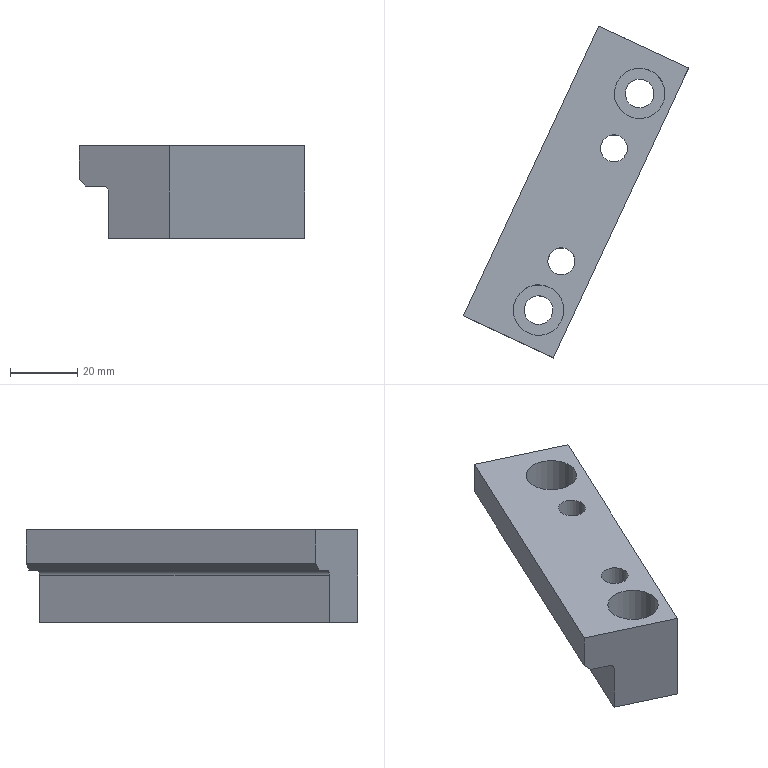Part | STEP file | gslz 2016.10.28-13_id1470_x_t | 1 solid | 18 faces | box 66.885 x 98.566 x 27.5 mm | volume 53451 mm3 | plane 11 | cylinder 7 | commonest cylinder face diameters 8 x2 8.5 x2 15 x2 3 x1
STEP:
#1=CARTESIAN_POINT('',(0.,0.,0.));
#2=DIRECTION('',(0.,0.,1.));
#3=DIRECTION('',(1.,0.,0.));
#4=AXIS2_PLACEMENT_3D('',#1,#2,#3);
#5=CARTESIAN_POINT('',(847.733,-374.977,-63.5));
#6=VERTEX_POINT('',#5);
#7=CARTESIAN_POINT('',(845.921,-374.132,-61.5));
#8=VERTEX_POINT('',#7);
#9=CARTESIAN_POINT('',(845.921,-374.132,-61.5));
#10=DIRECTION('',(-0.6409,0.2988,0.7071));
#11=VECTOR('',#10,1.);
#12=LINE('',#9,#11);
#13=CARTESIAN_POINT('',(867.052,-328.817,-61.5));
#14=DIRECTION('',(-0.6409,0.2988,-0.7071));
#15=DIRECTION('',(-0.2793,0.7673,0.5774));
#16=AXIS2_PLACEMENT_3D('',#13,#14,#15);
#17=PLANE('',#16);
#18=CARTESIAN_POINT('',(-28.868,-40.825));
#19=DIRECTION('',(0.8165,-0.5774));
#20=VECTOR('',#19,1.);
#21=LINE('',#18,#20);
#22=(GEOMETRIC_REPRESENTATION_CONTEXT(2)PARAMETRIC_REPRESENTATION_CONTEXT()REPRESENTATION_CONTEXT('',''));
#23=DEFINITIONAL_REPRESENTATION('',(#21),#22);
#24=PCURVE('',#17,#23);
#25=CARTESIAN_POINT('',(872.657,-386.599,-79.639));
#26=DIRECTION('',(0.4226,0.9063,0.));
#27=DIRECTION('',(0.9063,-0.4226,0.));
#28=AXIS2_PLACEMENT_3D('',#25,#26,#27);
#29=PLANE('',#28);
#30=CARTESIAN_POINT('',(-29.5,-18.139));
#31=DIRECTION('',(-0.7071,-0.7071));
#32=VECTOR('',#31,1.);
#33=LINE('',#30,#32);
#34=(GEOMETRIC_REPRESENTATION_CONTEXT(2)PARAMETRIC_REPRESENTATION_CONTEXT()REPRESENTATION_CONTEXT('',''));
#35=DEFINITIONAL_REPRESENTATION('',(#33),#34);
#36=PCURVE('',#29,#35);
#37=SURFACE_CURVE('',#12,(#24,#36),.PCURVE_S1.);
#38=EDGE_CURVE('',#6,#8,#37,.T.);
#39=ORIENTED_EDGE('',*,*,#38,.T.);
#40=CARTESIAN_POINT('',(886.069,-288.033,-61.5));
#41=VERTEX_POINT('',#40);
#42=CARTESIAN_POINT('',(867.052,-328.817,-61.5));
#43=DIRECTION('',(0.4226,0.9063,0.));
#44=VECTOR('',#43,1.);
#45=LINE('',#42,#44);
#46=CARTESIAN_POINT('',(0.,0.));
#47=DIRECTION('',(0.5774,0.8165));
#48=VECTOR('',#47,1.);
#49=LINE('',#46,#48);
#50=(GEOMETRIC_REPRESENTATION_CONTEXT(2)PARAMETRIC_REPRESENTATION_CONTEXT()REPRESENTATION_CONTEXT('',''));
#51=DEFINITIONAL_REPRESENTATION('',(#49),#50);
#52=PCURVE('',#17,#51);
#53=CARTESIAN_POINT('',(867.052,-328.817,-51.5));
#54=DIRECTION('',(0.9063,-0.4226,0.));
#55=DIRECTION('',(-0.4226,-0.9063,0.));
#56=AXIS2_PLACEMENT_3D('',#53,#54,#55);
#57=PLANE('',#56);
#58=CARTESIAN_POINT('',(0.,10.));
#59=DIRECTION('',(-1.,0.));
#60=VECTOR('',#59,1.);
#61=LINE('',#58,#60);
#62=(GEOMETRIC_REPRESENTATION_CONTEXT(2)PARAMETRIC_REPRESENTATION_CONTEXT()REPRESENTATION_CONTEXT('',''));
#63=DEFINITIONAL_REPRESENTATION('',(#61),#62);
#64=PCURVE('',#57,#63);
#65=SURFACE_CURVE('',#45,(#52,#64),.PCURVE_S1.);
#66=EDGE_CURVE('',#8,#41,#65,.T.);
#67=ORIENTED_EDGE('',*,*,#66,.T.);
#68=CARTESIAN_POINT('',(887.882,-288.878,-63.5));
#69=VERTEX_POINT('',#68);
#70=CARTESIAN_POINT('',(907.657,-298.1,-85.32));
#71=DIRECTION('',(0.6409,-0.2988,-0.7071));
#72=VECTOR('',#71,1.);
#73=LINE('',#70,#72);
#74=CARTESIAN_POINT('',(-1.524,56.191));
#75=DIRECTION('',(-0.8165,0.5774));
#76=VECTOR('',#75,1.);
#77=LINE('',#74,#76);
#78=(GEOMETRIC_REPRESENTATION_CONTEXT(2)PARAMETRIC_REPRESENTATION_CONTEXT()REPRESENTATION_CONTEXT('',''));
#79=DEFINITIONAL_REPRESENTATION('',(#77),#78);
#80=PCURVE('',#17,#79);
#81=CARTESIAN_POINT('',(912.805,-300.5,-79.639));
#82=DIRECTION('',(0.4226,0.9063,0.));
#83=DIRECTION('',(0.9063,-0.4226,0.));
#84=AXIS2_PLACEMENT_3D('',#81,#82,#83);
#85=PLANE('',#84);
#86=CARTESIAN_POINT('',(-5.68,5.68));
#87=DIRECTION('',(0.7071,0.7071));
#88=VECTOR('',#87,1.);
#89=LINE('',#86,#88);
#90=(GEOMETRIC_REPRESENTATION_CONTEXT(2)PARAMETRIC_REPRESENTATION_CONTEXT()REPRESENTATION_CONTEXT('',''));
#91=DEFINITIONAL_REPRESENTATION('',(#89),#90);
#92=PCURVE('',#85,#91);
#93=SURFACE_CURVE('',#73,(#80,#92),.PCURVE_S1.);
#94=EDGE_CURVE('',#41,#69,#93,.T.);
#95=ORIENTED_EDGE('',*,*,#94,.T.);
#96=CARTESIAN_POINT('',(868.864,-329.662,-63.5));
#97=DIRECTION('',(-0.4226,-0.9063,0.));
#98=VECTOR('',#97,1.);
#99=LINE('',#96,#98);
#100=CARTESIAN_POINT('',(-2.309,1.633));
#101=DIRECTION('',(-0.5774,-0.8165));
#102=VECTOR('',#101,1.);
#103=LINE('',#100,#102);
#104=(GEOMETRIC_REPRESENTATION_CONTEXT(2)PARAMETRIC_REPRESENTATION_CONTEXT()REPRESENTATION_CONTEXT('',''));
#105=DEFINITIONAL_REPRESENTATION('',(#103),#104);
#106=PCURVE('',#17,#105);
#107=CARTESIAN_POINT('',(893.788,-341.284,-63.5));
#108=DIRECTION('',(0.,0.,-1.));
#109=DIRECTION('',(-0.342,0.9397,0.));
#110=AXIS2_PLACEMENT_3D('',#107,#108,#109);
#111=PLANE('',#110);
#112=CARTESIAN_POINT('',(19.445,-19.445));
#113=DIRECTION('',(-0.7071,-0.7071));
#114=VECTOR('',#113,1.);
#115=LINE('',#112,#114);
#116=(GEOMETRIC_REPRESENTATION_CONTEXT(2)PARAMETRIC_REPRESENTATION_CONTEXT()REPRESENTATION_CONTEXT('',''));
#117=DEFINITIONAL_REPRESENTATION('',(#115),#116);
#118=PCURVE('',#111,#117);
#119=SURFACE_CURVE('',#99,(#106,#118),.PCURVE_S1.);
#120=EDGE_CURVE('',#69,#6,#119,.T.);
#121=ORIENTED_EDGE('',*,*,#120,.T.);
#122=EDGE_LOOP('',(#39,#67,#95,#121));
#123=FACE_BOUND('',#122,.T.);
#124=ADVANCED_FACE('',(#123),#17,.T.);
#125=CARTESIAN_POINT('',(893.32,-291.414,-63.5));
#126=VERTEX_POINT('',#125);
#127=CARTESIAN_POINT('',(912.805,-300.5,-63.5));
#128=DIRECTION('',(-0.9063,0.4226,0.));
#129=VECTOR('',#128,1.);
#130=LINE('',#127,#129);
#131=CARTESIAN_POINT('',(31.82,31.82));
#132=DIRECTION('',(0.7071,-0.7071));
#133=VECTOR('',#132,1.);
#134=LINE('',#131,#133);
#135=(GEOMETRIC_REPRESENTATION_CONTEXT(2)PARAMETRIC_REPRESENTATION_CONTEXT()REPRESENTATION_CONTEXT('',''));
#136=DEFINITIONAL_REPRESENTATION('',(#134),#135);
#137=PCURVE('',#111,#136);
#138=CARTESIAN_POINT('',(0.,-16.139));
#139=DIRECTION('',(-1.,0.));
#140=VECTOR('',#139,1.);
#141=LINE('',#138,#140);
#142=(GEOMETRIC_REPRESENTATION_CONTEXT(2)PARAMETRIC_REPRESENTATION_CONTEXT()REPRESENTATION_CONTEXT('',''));
#143=DEFINITIONAL_REPRESENTATION('',(#141),#142);
#144=PCURVE('',#85,#143);
#145=SURFACE_CURVE('',#130,(#137,#144),.PCURVE_S1.);
#146=EDGE_CURVE('',#126,#69,#145,.T.);
#147=ORIENTED_EDGE('',*,*,#146,.F.);
#148=CARTESIAN_POINT('',(853.171,-377.513,-63.5));
#149=VERTEX_POINT('',#148);
#150=CARTESIAN_POINT('',(874.302,-332.198,-63.5));
#151=DIRECTION('',(0.4226,0.9063,0.));
#152=VECTOR('',#151,1.);
#153=LINE('',#150,#152);
#154=CARTESIAN_POINT('',(15.203,-15.203));
#155=DIRECTION('',(0.7071,0.7071));
#156=VECTOR('',#155,1.);
#157=LINE('',#154,#156);
#158=(GEOMETRIC_REPRESENTATION_CONTEXT(2)PARAMETRIC_REPRESENTATION_CONTEXT()REPRESENTATION_CONTEXT('',''));
#159=DEFINITIONAL_REPRESENTATION('',(#157),#158);
#160=PCURVE('',#111,#159);
#161=CARTESIAN_POINT('',(874.302,-332.198,-65.));
#162=DIRECTION('',(0.4226,0.9063,0.));
#163=DIRECTION('',(0.9063,-0.4226,0.));
#164=AXIS2_PLACEMENT_3D('',#161,#162,#163);
#165=CYLINDRICAL_SURFACE('',#164,1.5);
#166=CARTESIAN_POINT('',(4.712,0.));
#167=DIRECTION('',(0.,1.));
#168=VECTOR('',#167,1.);
#169=LINE('',#166,#168);
#170=(GEOMETRIC_REPRESENTATION_CONTEXT(2)PARAMETRIC_REPRESENTATION_CONTEXT()REPRESENTATION_CONTEXT('',''));
#171=DEFINITIONAL_REPRESENTATION('',(#169),#170);
#172=PCURVE('',#165,#171);
#173=SURFACE_CURVE('',#153,(#160,#172),.PCURVE_S1.);
#174=EDGE_CURVE('',#149,#126,#173,.T.);
#175=ORIENTED_EDGE('',*,*,#174,.F.);
#176=CARTESIAN_POINT('',(872.657,-386.599,-63.5));
#177=DIRECTION('',(-0.9063,0.4226,0.));
#178=VECTOR('',#177,1.);
#179=LINE('',#176,#178);
#180=CARTESIAN_POINT('',(-35.355,-35.355));
#181=DIRECTION('',(0.7071,-0.7071));
#182=VECTOR('',#181,1.);
#183=LINE('',#180,#182);
#184=(GEOMETRIC_REPRESENTATION_CONTEXT(2)PARAMETRIC_REPRESENTATION_CONTEXT()REPRESENTATION_CONTEXT('',''));
#185=DEFINITIONAL_REPRESENTATION('',(#183),#184);
#186=PCURVE('',#111,#185);
#187=CARTESIAN_POINT('',(0.,-16.139));
#188=DIRECTION('',(-1.,0.));
#189=VECTOR('',#188,1.);
#190=LINE('',#187,#189);
#191=(GEOMETRIC_REPRESENTATION_CONTEXT(2)PARAMETRIC_REPRESENTATION_CONTEXT()REPRESENTATION_CONTEXT('',''));
#192=DEFINITIONAL_REPRESENTATION('',(#190),#191);
#193=PCURVE('',#29,#192);
#194=SURFACE_CURVE('',#179,(#186,#193),.PCURVE_S1.);
#195=EDGE_CURVE('',#149,#6,#194,.T.);
#196=ORIENTED_EDGE('',*,*,#195,.T.);
#197=ORIENTED_EDGE('',*,*,#120,.F.);
#198=EDGE_LOOP('',(#147,#175,#196,#197));
#199=FACE_BOUND('',#198,.T.);
#200=ADVANCED_FACE('',(#199),#111,.T.);
#201=CARTESIAN_POINT('',(894.679,-292.048,-65.));
#202=VERTEX_POINT('',#201);
#203=CARTESIAN_POINT('',(854.531,-378.147,-65.));
#204=VERTEX_POINT('',#203);
#205=CARTESIAN_POINT('',(875.661,-332.832,-65.));
#206=DIRECTION('',(-0.4226,-0.9063,0.));
#207=VECTOR('',#206,1.);
#208=LINE('',#205,#207);
#209=CARTESIAN_POINT('',(6.283,0.));
#210=DIRECTION('',(0.,-1.));
#211=VECTOR('',#210,1.);
#212=LINE('',#209,#211);
#213=(GEOMETRIC_REPRESENTATION_CONTEXT(2)PARAMETRIC_REPRESENTATION_CONTEXT()REPRESENTATION_CONTEXT('',''));
#214=DEFINITIONAL_REPRESENTATION('',(#212),#213);
#215=PCURVE('',#165,#214);
#216=CARTESIAN_POINT('',(875.661,-332.832,-79.639));
#217=DIRECTION('',(0.9063,-0.4226,0.));
#218=DIRECTION('',(-0.4226,-0.9063,0.));
#219=AXIS2_PLACEMENT_3D('',#216,#217,#218);
#220=PLANE('',#219);
#221=CARTESIAN_POINT('',(0.,-14.639));
#222=DIRECTION('',(1.,0.));
#223=VECTOR('',#222,1.);
#224=LINE('',#221,#223);
#225=(GEOMETRIC_REPRESENTATION_CONTEXT(2)PARAMETRIC_REPRESENTATION_CONTEXT()REPRESENTATION_CONTEXT('',''));
#226=DEFINITIONAL_REPRESENTATION('',(#224),#225);
#227=PCURVE('',#220,#226);
#228=SURFACE_CURVE('',#208,(#215,#227),.PCURVE_S1.);
#229=EDGE_CURVE('',#202,#204,#228,.T.);
#230=ORIENTED_EDGE('',*,*,#229,.F.);
#231=CARTESIAN_POINT('',(893.32,-291.414,-65.));
#232=DIRECTION('',(0.4226,0.9063,0.));
#233=DIRECTION('',(0.9063,-0.4226,0.));
#234=AXIS2_PLACEMENT_3D('',#231,#232,#233);
#235=CIRCLE('',#234,1.5);
#236=CARTESIAN_POINT('',(0.,45.));
#237=DIRECTION('',(1.,0.));
#238=VECTOR('',#237,1.);
#239=LINE('',#236,#238);
#240=(GEOMETRIC_REPRESENTATION_CONTEXT(2)PARAMETRIC_REPRESENTATION_CONTEXT()REPRESENTATION_CONTEXT('',''));
#241=DEFINITIONAL_REPRESENTATION('',(#239),#240);
#242=PCURVE('',#165,#241);
#243=CARTESIAN_POINT('',(-21.5,-14.639));
#244=DIRECTION('',(1.,0.));
#245=AXIS2_PLACEMENT_2D('',#243,#244);
#246=CIRCLE('',#245,1.5);
#247=(GEOMETRIC_REPRESENTATION_CONTEXT(2)PARAMETRIC_REPRESENTATION_CONTEXT()REPRESENTATION_CONTEXT('',''));
#248=DEFINITIONAL_REPRESENTATION('',(#246),#247);
#249=PCURVE('',#85,#248);
#250=SURFACE_CURVE('',#235,(#242,#249),.PCURVE_S1.);
#251=EDGE_CURVE('',#126,#202,#250,.T.);
#252=ORIENTED_EDGE('',*,*,#251,.F.);
#253=ORIENTED_EDGE('',*,*,#174,.F.);
#254=CARTESIAN_POINT('',(853.171,-377.513,-65.));
#255=DIRECTION('',(-0.4226,-0.9063,0.));
#256=DIRECTION('',(0.9063,-0.4226,0.));
#257=AXIS2_PLACEMENT_3D('',#254,#255,#256);
#258=CIRCLE('',#257,1.5);
#259=CARTESIAN_POINT('',(6.283,-50.));
#260=DIRECTION('',(-1.,0.));
#261=VECTOR('',#260,1.);
#262=LINE('',#259,#261);
#263=(GEOMETRIC_REPRESENTATION_CONTEXT(2)PARAMETRIC_REPRESENTATION_CONTEXT()REPRESENTATION_CONTEXT('',''));
#264=DEFINITIONAL_REPRESENTATION('',(#262),#263);
#265=PCURVE('',#165,#264);
#266=CARTESIAN_POINT('',(-20.,-14.639));
#267=CARTESIAN_POINT('',(-20.,-17.237));
#268=CARTESIAN_POINT('',(-22.25,-15.938));
#269=CARTESIAN_POINT('',(-24.5,-14.639));
#270=CARTESIAN_POINT('',(-22.25,-13.34));
#271=CARTESIAN_POINT('',(-20.,-12.041));
#272=CARTESIAN_POINT('',(-20.,-14.639));
#273=(BOUNDED_CURVE()B_SPLINE_CURVE(2,(#266,#267,#268,#269,#270,#271,#272),.UNSPECIFIED.,.T.,.F.)B_SPLINE_CURVE_WITH_KNOTS((1,2,2,2,2,1),(-2.094,0.,2.094,4.189,6.283,8.378),.UNSPECIFIED.)CURVE()GEOMETRIC_REPRESENTATION_ITEM()RATIONAL_B_SPLINE_CURVE((1.,0.5,1.,0.5,1.,0.5,1.))REPRESENTATION_ITEM(''));
#274=(GEOMETRIC_REPRESENTATION_CONTEXT(2)PARAMETRIC_REPRESENTATION_CONTEXT()REPRESENTATION_CONTEXT('',''));
#275=DEFINITIONAL_REPRESENTATION('',(#273),#274);
#276=PCURVE('',#29,#275);
#277=SURFACE_CURVE('',#258,(#265,#276),.PCURVE_S1.);
#278=EDGE_CURVE('',#204,#149,#277,.T.);
#279=ORIENTED_EDGE('',*,*,#278,.F.);
#280=EDGE_LOOP('',(#230,#252,#253,#279));
#281=FACE_BOUND('',#280,.F.);
#282=ADVANCED_FACE('',(#281),#165,.F.);
#283=CARTESIAN_POINT('',(896.795,-304.062,-66.5));
#284=VERTEX_POINT('',#283);
#285=CARTESIAN_POINT('',(898.248,-308.056,-66.5));
#286=DIRECTION('',(0.,0.,-1.));
#287=DIRECTION('',(-0.342,0.9397,0.));
#288=AXIS2_PLACEMENT_3D('',#285,#286,#287);
#289=CIRCLE('',#288,4.25);
#290=CARTESIAN_POINT('',(898.248,-308.056,-66.5));
#291=DIRECTION('',(0.,0.,-1.));
#292=DIRECTION('',(-0.342,0.9397,0.));
#293=AXIS2_PLACEMENT_3D('',#290,#291,#292);
#294=PLANE('',#293);
#295=CARTESIAN_POINT('',(0.,0.));
#296=DIRECTION('',(1.,0.));
#297=AXIS2_PLACEMENT_2D('',#295,#296);
#298=CIRCLE('',#297,4.25);
#299=(GEOMETRIC_REPRESENTATION_CONTEXT(2)PARAMETRIC_REPRESENTATION_CONTEXT()REPRESENTATION_CONTEXT('',''));
#300=DEFINITIONAL_REPRESENTATION('',(#298),#299);
#301=PCURVE('',#294,#300);
#302=CARTESIAN_POINT('',(898.248,-308.056,-101.5));
#303=DIRECTION('',(0.,0.,-1.));
#304=DIRECTION('',(-0.342,0.9397,0.));
#305=AXIS2_PLACEMENT_3D('',#302,#303,#304);
#306=CYLINDRICAL_SURFACE('',#305,4.25);
#307=CARTESIAN_POINT('',(0.,-35.));
#308=DIRECTION('',(1.,0.));
#309=VECTOR('',#308,1.);
#310=LINE('',#307,#309);
#311=(GEOMETRIC_REPRESENTATION_CONTEXT(2)PARAMETRIC_REPRESENTATION_CONTEXT()REPRESENTATION_CONTEXT('',''));
#312=DEFINITIONAL_REPRESENTATION('',(#310),#311);
#313=PCURVE('',#306,#312);
#314=SURFACE_CURVE('',#289,(#301,#313),.PCURVE_S1.);
#315=EDGE_CURVE('',#284,#284,#314,.T.);
#316=ORIENTED_EDGE('',*,*,#315,.T.);
#317=EDGE_LOOP('',(#316));
#318=FACE_BOUND('',#317,.T.);
#319=CARTESIAN_POINT('',(895.683,-301.008,-66.5));
#320=VERTEX_POINT('',#319);
#321=CARTESIAN_POINT('',(898.248,-308.056,-66.5));
#322=DIRECTION('',(0.,0.,-1.));
#323=DIRECTION('',(-0.342,0.9397,0.));
#324=AXIS2_PLACEMENT_3D('',#321,#322,#323);
#325=CIRCLE('',#324,7.5);
#326=CARTESIAN_POINT('',(0.,0.));
#327=DIRECTION('',(1.,0.));
#328=AXIS2_PLACEMENT_2D('',#326,#327);
#329=CIRCLE('',#328,7.5);
#330=(GEOMETRIC_REPRESENTATION_CONTEXT(2)PARAMETRIC_REPRESENTATION_CONTEXT()REPRESENTATION_CONTEXT('',''));
#331=DEFINITIONAL_REPRESENTATION('',(#329),#330);
#332=PCURVE('',#294,#331);
#333=CARTESIAN_POINT('',(898.248,-308.056,-51.5));
#334=DIRECTION('',(0.,0.,-1.));
#335=DIRECTION('',(-0.342,0.9397,0.));
#336=AXIS2_PLACEMENT_3D('',#333,#334,#335);
#337=CYLINDRICAL_SURFACE('',#336,7.5);
#338=CARTESIAN_POINT('',(0.,15.));
#339=DIRECTION('',(1.,0.));
#340=VECTOR('',#339,1.);
#341=LINE('',#338,#340);
#342=(GEOMETRIC_REPRESENTATION_CONTEXT(2)PARAMETRIC_REPRESENTATION_CONTEXT()REPRESENTATION_CONTEXT('',''));
#343=DEFINITIONAL_REPRESENTATION('',(#341),#342);
#344=PCURVE('',#337,#343);
#345=SURFACE_CURVE('',#325,(#332,#344),.PCURVE_S1.);
#346=EDGE_CURVE('',#320,#320,#345,.T.);
#347=ORIENTED_EDGE('',*,*,#346,.F.);
#348=EDGE_LOOP('',(#347));
#349=FACE_BOUND('',#348,.T.);
#350=ADVANCED_FACE('',(#318,#349),#294,.F.);
#351=CARTESIAN_POINT('',(866.789,-368.41,-66.5));
#352=VERTEX_POINT('',#351);
#353=CARTESIAN_POINT('',(868.242,-372.404,-66.5));
#354=DIRECTION('',(0.,0.,-1.));
#355=DIRECTION('',(-0.342,0.9397,0.));
#356=AXIS2_PLACEMENT_3D('',#353,#354,#355);
#357=CIRCLE('',#356,4.25);
#358=CARTESIAN_POINT('',(874.582,-358.809,-66.5));
#359=DIRECTION('',(0.,0.,-1.));
#360=DIRECTION('',(-0.342,0.9397,0.));
#361=AXIS2_PLACEMENT_3D('',#358,#359,#360);
#362=PLANE('',#361);
#363=CARTESIAN_POINT('',(-10.607,-10.607));
#364=DIRECTION('',(1.,0.));
#365=AXIS2_PLACEMENT_2D('',#363,#364);
#366=CIRCLE('',#365,4.25);
#367=(GEOMETRIC_REPRESENTATION_CONTEXT(2)PARAMETRIC_REPRESENTATION_CONTEXT()REPRESENTATION_CONTEXT('',''));
#368=DEFINITIONAL_REPRESENTATION('',(#366),#367);
#369=PCURVE('',#362,#368);
#370=CARTESIAN_POINT('',(868.242,-372.404,-101.5));
#371=DIRECTION('',(0.,0.,-1.));
#372=DIRECTION('',(-0.342,0.9397,0.));
#373=AXIS2_PLACEMENT_3D('',#370,#371,#372);
#374=CYLINDRICAL_SURFACE('',#373,4.25);
#375=CARTESIAN_POINT('',(0.,-35.));
#376=DIRECTION('',(1.,0.));
#377=VECTOR('',#376,1.);
#378=LINE('',#375,#377);
#379=(GEOMETRIC_REPRESENTATION_CONTEXT(2)PARAMETRIC_REPRESENTATION_CONTEXT()REPRESENTATION_CONTEXT('',''));
#380=DEFINITIONAL_REPRESENTATION('',(#378),#379);
#381=PCURVE('',#374,#380);
#382=SURFACE_CURVE('',#357,(#369,#381),.PCURVE_S1.);
#383=EDGE_CURVE('',#352,#352,#382,.T.);
#384=ORIENTED_EDGE('',*,*,#383,.T.);
#385=EDGE_LOOP('',(#384));
#386=FACE_BOUND('',#385,.T.);
#387=CARTESIAN_POINT('',(865.677,-365.356,-66.5));
#388=VERTEX_POINT('',#387);
#389=CARTESIAN_POINT('',(868.242,-372.404,-66.5));
#390=DIRECTION('',(0.,0.,-1.));
#391=DIRECTION('',(-0.342,0.9397,0.));
#392=AXIS2_PLACEMENT_3D('',#389,#390,#391);
#393=CIRCLE('',#392,7.5);
#394=CARTESIAN_POINT('',(-10.607,-10.607));
#395=DIRECTION('',(1.,0.));
#396=AXIS2_PLACEMENT_2D('',#394,#395);
#397=CIRCLE('',#396,7.5);
#398=(GEOMETRIC_REPRESENTATION_CONTEXT(2)PARAMETRIC_REPRESENTATION_CONTEXT()REPRESENTATION_CONTEXT('',''));
#399=DEFINITIONAL_REPRESENTATION('',(#397),#398);
#400=PCURVE('',#362,#399);
#401=CARTESIAN_POINT('',(868.242,-372.404,-51.5));
#402=DIRECTION('',(0.,0.,-1.));
#403=DIRECTION('',(-0.342,0.9397,0.));
#404=AXIS2_PLACEMENT_3D('',#401,#402,#403);
#405=CYLINDRICAL_SURFACE('',#404,7.5);
#406=CARTESIAN_POINT('',(0.,15.));
#407=DIRECTION('',(1.,0.));
#408=VECTOR('',#407,1.);
#409=LINE('',#406,#408);
#410=(GEOMETRIC_REPRESENTATION_CONTEXT(2)PARAMETRIC_REPRESENTATION_CONTEXT()REPRESENTATION_CONTEXT('',''));
#411=DEFINITIONAL_REPRESENTATION('',(#409),#410);
#412=PCURVE('',#405,#411);
#413=SURFACE_CURVE('',#393,(#400,#412),.PCURVE_S1.);
#414=EDGE_CURVE('',#388,#388,#413,.T.);
#415=ORIENTED_EDGE('',*,*,#414,.F.);
#416=EDGE_LOOP('',(#415));
#417=FACE_BOUND('',#416,.T.);
#418=ADVANCED_FACE('',(#386,#417),#362,.F.);
#419=CARTESIAN_POINT('',(886.069,-288.033,-51.5));
#420=VERTEX_POINT('',#419);
#421=CARTESIAN_POINT('',(886.069,-288.033,-51.5));
#422=DIRECTION('',(0.,0.,-1.));
#423=VECTOR('',#422,1.);
#424=LINE('',#421,#423);
#425=CARTESIAN_POINT('',(-45.,0.));
#426=DIRECTION('',(0.,1.));
#427=VECTOR('',#426,1.);
#428=LINE('',#425,#427);
#429=(GEOMETRIC_REPRESENTATION_CONTEXT(2)PARAMETRIC_REPRESENTATION_CONTEXT()REPRESENTATION_CONTEXT('',''));
#430=DEFINITIONAL_REPRESENTATION('',(#428),#429);
#431=PCURVE('',#57,#430);
#432=CARTESIAN_POINT('',(-29.5,-28.139));
#433=DIRECTION('',(0.,1.));
#434=VECTOR('',#433,1.);
#435=LINE('',#432,#434);
#436=(GEOMETRIC_REPRESENTATION_CONTEXT(2)PARAMETRIC_REPRESENTATION_CONTEXT()REPRESENTATION_CONTEXT('',''));
#437=DEFINITIONAL_REPRESENTATION('',(#435),#436);
#438=PCURVE('',#85,#437);
#439=SURFACE_CURVE('',#424,(#431,#438),.PCURVE_S1.);
#440=EDGE_CURVE('',#420,#41,#439,.T.);
#441=ORIENTED_EDGE('',*,*,#440,.T.);
#442=ORIENTED_EDGE('',*,*,#66,.F.);
#443=CARTESIAN_POINT('',(845.921,-374.132,-51.5));
#444=VERTEX_POINT('',#443);
#445=CARTESIAN_POINT('',(845.921,-374.132,-51.5));
#446=DIRECTION('',(0.,0.,-1.));
#447=VECTOR('',#446,1.);
#448=LINE('',#445,#447);
#449=CARTESIAN_POINT('',(50.,0.));
#450=DIRECTION('',(0.,1.));
#451=VECTOR('',#450,1.);
#452=LINE('',#449,#451);
#453=(GEOMETRIC_REPRESENTATION_CONTEXT(2)PARAMETRIC_REPRESENTATION_CONTEXT()REPRESENTATION_CONTEXT('',''));
#454=DEFINITIONAL_REPRESENTATION('',(#452),#453);
#455=PCURVE('',#57,#454);
#456=CARTESIAN_POINT('',(-29.5,-28.139));
#457=DIRECTION('',(0.,1.));
#458=VECTOR('',#457,1.);
#459=LINE('',#456,#458);
#460=(GEOMETRIC_REPRESENTATION_CONTEXT(2)PARAMETRIC_REPRESENTATION_CONTEXT()REPRESENTATION_CONTEXT('',''));
#461=DEFINITIONAL_REPRESENTATION('',(#459),#460);
#462=PCURVE('',#29,#461);
#463=SURFACE_CURVE('',#448,(#455,#462),.PCURVE_S1.);
#464=EDGE_CURVE('',#444,#8,#463,.T.);
#465=ORIENTED_EDGE('',*,*,#464,.F.);
#466=CARTESIAN_POINT('',(867.052,-328.817,-51.5));
#467=DIRECTION('',(-0.4226,-0.9063,0.));
#468=VECTOR('',#467,1.);
#469=LINE('',#466,#468);
#470=CARTESIAN_POINT('',(0.,0.));
#471=DIRECTION('',(1.,0.));
#472=VECTOR('',#471,1.);
#473=LINE('',#470,#472);
#474=(GEOMETRIC_REPRESENTATION_CONTEXT(2)PARAMETRIC_REPRESENTATION_CONTEXT()REPRESENTATION_CONTEXT('',''));
#475=DEFINITIONAL_REPRESENTATION('',(#473),#474);
#476=PCURVE('',#57,#475);
#477=CARTESIAN_POINT('',(893.788,-341.284,-51.5));
#478=DIRECTION('',(0.,0.,-1.));
#479=DIRECTION('',(-0.342,0.9397,0.));
#480=AXIS2_PLACEMENT_3D('',#477,#478,#479);
#481=PLANE('',#480);
#482=CARTESIAN_POINT('',(20.86,-20.86));
#483=DIRECTION('',(-0.7071,-0.7071));
#484=VECTOR('',#483,1.);
#485=LINE('',#482,#484);
#486=(GEOMETRIC_REPRESENTATION_CONTEXT(2)PARAMETRIC_REPRESENTATION_CONTEXT()REPRESENTATION_CONTEXT('',''));
#487=DEFINITIONAL_REPRESENTATION('',(#485),#486);
#488=PCURVE('',#481,#487);
#489=SURFACE_CURVE('',#469,(#476,#488),.PCURVE_S1.);
#490=EDGE_CURVE('',#420,#444,#489,.T.);
#491=ORIENTED_EDGE('',*,*,#490,.F.);
#492=EDGE_LOOP('',(#441,#442,#465,#491));
#493=FACE_BOUND('',#492,.T.);
#494=ADVANCED_FACE('',(#493),#57,.F.);
#495=ORIENTED_EDGE('',*,*,#346,.F.);
#496=CARTESIAN_POINT('',(895.683,-301.008,-51.5));
#497=VERTEX_POINT('',#496);
#498=CARTESIAN_POINT('',(895.683,-301.008,-51.5));
#499=CARTESIAN_POINT('',(895.683,-301.008,-66.5));
#500=B_SPLINE_CURVE_WITH_KNOTS('',1,(#498,#499),.UNSPECIFIED.,.F.,.F.,(2,2),(0.,15.),.PIECEWISE_BEZIER_KNOTS.);
#501=CARTESIAN_POINT('',(0.,0.));
#502=DIRECTION('',(0.,1.));
#503=VECTOR('',#502,1.);
#504=LINE('',#501,#503);
#505=(GEOMETRIC_REPRESENTATION_CONTEXT(2)PARAMETRIC_REPRESENTATION_CONTEXT()REPRESENTATION_CONTEXT('',''));
#506=DEFINITIONAL_REPRESENTATION('',(#504),#505);
#507=PCURVE('',#337,#506);
#508=CARTESIAN_POINT('',(6.283,0.));
#509=DIRECTION('',(0.,1.));
#510=VECTOR('',#509,1.);
#511=LINE('',#508,#510);
#512=(GEOMETRIC_REPRESENTATION_CONTEXT(2)PARAMETRIC_REPRESENTATION_CONTEXT()REPRESENTATION_CONTEXT('',''));
#513=DEFINITIONAL_REPRESENTATION('',(#511),#512);
#514=PCURVE('',#337,#513);
#515=SEAM_CURVE('',#500,(#507,#514),.PCURVE_S1.);
#516=EDGE_CURVE('',#497,#320,#515,.T.);
#517=ORIENTED_EDGE('',*,*,#516,.F.);
#518=CARTESIAN_POINT('',(898.248,-308.056,-51.5));
#519=DIRECTION('',(0.,0.,1.));
#520=DIRECTION('',(-0.342,0.9397,0.));
#521=AXIS2_PLACEMENT_3D('',#518,#519,#520);
#522=CIRCLE('',#521,7.5);
#523=CARTESIAN_POINT('',(6.283,0.));
#524=DIRECTION('',(-1.,0.));
#525=VECTOR('',#524,1.);
#526=LINE('',#523,#525);
#527=(GEOMETRIC_REPRESENTATION_CONTEXT(2)PARAMETRIC_REPRESENTATION_CONTEXT()REPRESENTATION_CONTEXT('',''));
#528=DEFINITIONAL_REPRESENTATION('',(#526),#527);
#529=PCURVE('',#337,#528);
#530=CARTESIAN_POINT('',(37.198,15.556));
#531=CARTESIAN_POINT('',(37.198,2.566));
#532=CARTESIAN_POINT('',(25.948,9.061));
#533=CARTESIAN_POINT('',(14.698,15.556));
#534=CARTESIAN_POINT('',(25.948,22.052));
#535=CARTESIAN_POINT('',(37.198,28.547));
#536=CARTESIAN_POINT('',(37.198,15.556));
#537=(BOUNDED_CURVE()B_SPLINE_CURVE(2,(#530,#531,#532,#533,#534,#535,#536),.UNSPECIFIED.,.T.,.F.)B_SPLINE_CURVE_WITH_KNOTS((1,2,2,2,2,1),(-2.094,0.,2.094,4.189,6.283,8.378),.UNSPECIFIED.)CURVE()GEOMETRIC_REPRESENTATION_ITEM()RATIONAL_B_SPLINE_CURVE((1.,0.5,1.,0.5,1.,0.5,1.))REPRESENTATION_ITEM(''));
#538=(GEOMETRIC_REPRESENTATION_CONTEXT(2)PARAMETRIC_REPRESENTATION_CONTEXT()REPRESENTATION_CONTEXT('',''));
#539=DEFINITIONAL_REPRESENTATION('',(#537),#538);
#540=PCURVE('',#481,#539);
#541=SURFACE_CURVE('',#522,(#529,#540),.PCURVE_S1.);
#542=EDGE_CURVE('',#497,#497,#541,.T.);
#543=ORIENTED_EDGE('',*,*,#542,.F.);
#544=ORIENTED_EDGE('',*,*,#516,.T.);
#545=EDGE_LOOP('',(#495,#517,#543,#544));
#546=FACE_BOUND('',#545,.F.);
#547=ADVANCED_FACE('',(#546),#337,.F.);
#548=ORIENTED_EDGE('',*,*,#414,.F.);
#549=CARTESIAN_POINT('',(865.677,-365.356,-51.5));
#550=VERTEX_POINT('',#549);
#551=CARTESIAN_POINT('',(865.677,-365.356,-51.5));
#552=CARTESIAN_POINT('',(865.677,-365.356,-66.5));
#553=B_SPLINE_CURVE_WITH_KNOTS('',1,(#551,#552),.UNSPECIFIED.,.F.,.F.,(2,2),(0.,15.),.PIECEWISE_BEZIER_KNOTS.);
#554=CARTESIAN_POINT('',(0.,0.));
#555=DIRECTION('',(0.,1.));
#556=VECTOR('',#555,1.);
#557=LINE('',#554,#556);
#558=(GEOMETRIC_REPRESENTATION_CONTEXT(2)PARAMETRIC_REPRESENTATION_CONTEXT()REPRESENTATION_CONTEXT('',''));
#559=DEFINITIONAL_REPRESENTATION('',(#557),#558);
#560=PCURVE('',#405,#559);
#561=CARTESIAN_POINT('',(6.283,0.));
#562=DIRECTION('',(0.,1.));
#563=VECTOR('',#562,1.);
#564=LINE('',#561,#563);
#565=(GEOMETRIC_REPRESENTATION_CONTEXT(2)PARAMETRIC_REPRESENTATION_CONTEXT()REPRESENTATION_CONTEXT('',''));
#566=DEFINITIONAL_REPRESENTATION('',(#564),#565);
#567=PCURVE('',#405,#566);
#568=SEAM_CURVE('',#553,(#560,#567),.PCURVE_S1.);
#569=EDGE_CURVE('',#550,#388,#568,.T.);
#570=ORIENTED_EDGE('',*,*,#569,.F.);
#571=CARTESIAN_POINT('',(868.242,-372.404,-51.5));
#572=DIRECTION('',(0.,0.,1.));
#573=DIRECTION('',(-0.342,0.9397,0.));
#574=AXIS2_PLACEMENT_3D('',#571,#572,#573);
#575=CIRCLE('',#574,7.5);
#576=CARTESIAN_POINT('',(6.283,0.));
#577=DIRECTION('',(-1.,0.));
#578=VECTOR('',#577,1.);
#579=LINE('',#576,#578);
#580=(GEOMETRIC_REPRESENTATION_CONTEXT(2)PARAMETRIC_REPRESENTATION_CONTEXT()REPRESENTATION_CONTEXT('',''));
#581=DEFINITIONAL_REPRESENTATION('',(#579),#580);
#582=PCURVE('',#405,#581);
#583=CARTESIAN_POINT('',(-13.006,-34.648));
#584=CARTESIAN_POINT('',(-13.006,-47.639));
#585=CARTESIAN_POINT('',(-24.256,-41.143));
#586=CARTESIAN_POINT('',(-35.506,-34.648));
#587=CARTESIAN_POINT('',(-24.256,-28.153));
#588=CARTESIAN_POINT('',(-13.006,-21.658));
#589=CARTESIAN_POINT('',(-13.006,-34.648));
#590=(BOUNDED_CURVE()B_SPLINE_CURVE(2,(#583,#584,#585,#586,#587,#588,#589),.UNSPECIFIED.,.T.,.F.)B_SPLINE_CURVE_WITH_KNOTS((1,2,2,2,2,1),(-2.094,0.,2.094,4.189,6.283,8.378),.UNSPECIFIED.)CURVE()GEOMETRIC_REPRESENTATION_ITEM()RATIONAL_B_SPLINE_CURVE((1.,0.5,1.,0.5,1.,0.5,1.))REPRESENTATION_ITEM(''));
#591=(GEOMETRIC_REPRESENTATION_CONTEXT(2)PARAMETRIC_REPRESENTATION_CONTEXT()REPRESENTATION_CONTEXT('',''));
#592=DEFINITIONAL_REPRESENTATION('',(#590),#591);
#593=PCURVE('',#481,#592);
#594=SURFACE_CURVE('',#575,(#582,#593),.PCURVE_S1.);
#595=EDGE_CURVE('',#550,#550,#594,.T.);
#596=ORIENTED_EDGE('',*,*,#595,.F.);
#597=ORIENTED_EDGE('',*,*,#569,.T.);
#598=EDGE_LOOP('',(#548,#570,#596,#597));
#599=FACE_BOUND('',#598,.F.);
#600=ADVANCED_FACE('',(#599),#405,.F.);
#601=CARTESIAN_POINT('',(912.805,-300.5,-51.5));
#602=VERTEX_POINT('',#601);
#603=CARTESIAN_POINT('',(912.805,-300.5,-51.5));
#604=DIRECTION('',(-0.9063,0.4226,0.));
#605=VECTOR('',#604,1.);
#606=LINE('',#603,#605);
#607=CARTESIAN_POINT('',(0.,-28.139));
#608=DIRECTION('',(-1.,0.));
#609=VECTOR('',#608,1.);
#610=LINE('',#607,#609);
#611=(GEOMETRIC_REPRESENTATION_CONTEXT(2)PARAMETRIC_REPRESENTATION_CONTEXT()REPRESENTATION_CONTEXT('',''));
#612=DEFINITIONAL_REPRESENTATION('',(#610),#611);
#613=PCURVE('',#85,#612);
#614=CARTESIAN_POINT('',(31.82,31.82));
#615=DIRECTION('',(0.7071,-0.7071));
#616=VECTOR('',#615,1.);
#617=LINE('',#614,#616);
#618=(GEOMETRIC_REPRESENTATION_CONTEXT(2)PARAMETRIC_REPRESENTATION_CONTEXT()REPRESENTATION_CONTEXT('',''));
#619=DEFINITIONAL_REPRESENTATION('',(#617),#618);
#620=PCURVE('',#481,#619);
#621=SURFACE_CURVE('',#606,(#613,#620),.PCURVE_S1.);
#622=EDGE_CURVE('',#602,#420,#621,.T.);
#623=ORIENTED_EDGE('',*,*,#622,.F.);
#624=CARTESIAN_POINT('',(912.805,-300.5,-79.));
#625=VERTEX_POINT('',#624);
#626=CARTESIAN_POINT('',(912.805,-300.5,-79.639));
#627=DIRECTION('',(0.,0.,1.));
#628=VECTOR('',#627,1.);
#629=LINE('',#626,#628);
#630=CARTESIAN_POINT('',(0.,0.));
#631=DIRECTION('',(0.,-1.));
#632=VECTOR('',#631,1.);
#633=LINE('',#630,#632);
#634=(GEOMETRIC_REPRESENTATION_CONTEXT(2)PARAMETRIC_REPRESENTATION_CONTEXT()REPRESENTATION_CONTEXT('',''));
#635=DEFINITIONAL_REPRESENTATION('',(#633),#634);
#636=PCURVE('',#85,#635);
#637=CARTESIAN_POINT('',(893.788,-341.284,-79.639));
#638=DIRECTION('',(0.9063,-0.4226,0.));
#639=DIRECTION('',(-0.4226,-0.9063,0.));
#640=AXIS2_PLACEMENT_3D('',#637,#638,#639);
#641=PLANE('',#640);
#642=CARTESIAN_POINT('',(-45.,0.));
#643=DIRECTION('',(0.,-1.));
#644=VECTOR('',#643,1.);
#645=LINE('',#642,#644);
#646=(GEOMETRIC_REPRESENTATION_CONTEXT(2)PARAMETRIC_REPRESENTATION_CONTEXT()REPRESENTATION_CONTEXT('',''));
#647=DEFINITIONAL_REPRESENTATION('',(#645),#646);
#648=PCURVE('',#641,#647);
#649=SURFACE_CURVE('',#629,(#636,#648),.PCURVE_S1.);
#650=EDGE_CURVE('',#625,#602,#649,.T.);
#651=ORIENTED_EDGE('',*,*,#650,.F.);
#652=CARTESIAN_POINT('',(894.679,-292.048,-79.));
#653=VERTEX_POINT('',#652);
#654=CARTESIAN_POINT('',(912.805,-300.5,-79.));
#655=DIRECTION('',(-0.9063,0.4226,0.));
#656=VECTOR('',#655,1.);
#657=LINE('',#654,#656);
#658=CARTESIAN_POINT('',(0.,-0.6394));
#659=DIRECTION('',(-1.,0.));
#660=VECTOR('',#659,1.);
#661=LINE('',#658,#660);
#662=(GEOMETRIC_REPRESENTATION_CONTEXT(2)PARAMETRIC_REPRESENTATION_CONTEXT()REPRESENTATION_CONTEXT('',''));
#663=DEFINITIONAL_REPRESENTATION('',(#661),#662);
#664=PCURVE('',#85,#663);
#665=CARTESIAN_POINT('',(893.788,-341.284,-79.));
#666=DIRECTION('',(0.,0.,-1.));
#667=DIRECTION('',(-0.342,0.9397,0.));
#668=AXIS2_PLACEMENT_3D('',#665,#666,#667);
#669=PLANE('',#668);
#670=CARTESIAN_POINT('',(31.82,31.82));
#671=DIRECTION('',(0.7071,-0.7071));
#672=VECTOR('',#671,1.);
#673=LINE('',#670,#672);
#674=(GEOMETRIC_REPRESENTATION_CONTEXT(2)PARAMETRIC_REPRESENTATION_CONTEXT()REPRESENTATION_CONTEXT('',''));
#675=DEFINITIONAL_REPRESENTATION('',(#673),#674);
#676=PCURVE('',#669,#675);
#677=SURFACE_CURVE('',#657,(#664,#676),.PCURVE_S1.);
#678=EDGE_CURVE('',#625,#653,#677,.T.);
#679=ORIENTED_EDGE('',*,*,#678,.T.);
#680=CARTESIAN_POINT('',(894.679,-292.048,-79.639));
#681=DIRECTION('',(0.,0.,1.));
#682=VECTOR('',#681,1.);
#683=LINE('',#680,#682);
#684=CARTESIAN_POINT('',(-20.,0.));
#685=DIRECTION('',(0.,-1.));
#686=VECTOR('',#685,1.);
#687=LINE('',#684,#686);
#688=(GEOMETRIC_REPRESENTATION_CONTEXT(2)PARAMETRIC_REPRESENTATION_CONTEXT()REPRESENTATION_CONTEXT('',''));
#689=DEFINITIONAL_REPRESENTATION('',(#687),#688);
#690=PCURVE('',#85,#689);
#691=CARTESIAN_POINT('',(-45.,0.));
#692=DIRECTION('',(0.,-1.));
#693=VECTOR('',#692,1.);
#694=LINE('',#691,#693);
#695=(GEOMETRIC_REPRESENTATION_CONTEXT(2)PARAMETRIC_REPRESENTATION_CONTEXT()REPRESENTATION_CONTEXT('',''));
#696=DEFINITIONAL_REPRESENTATION('',(#694),#695);
#697=PCURVE('',#220,#696);
#698=SURFACE_CURVE('',#683,(#690,#697),.PCURVE_S1.);
#699=EDGE_CURVE('',#653,#202,#698,.T.);
#700=ORIENTED_EDGE('',*,*,#699,.T.);
#701=ORIENTED_EDGE('',*,*,#251,.F.);
#702=ORIENTED_EDGE('',*,*,#146,.T.);
#703=ORIENTED_EDGE('',*,*,#94,.F.);
#704=ORIENTED_EDGE('',*,*,#440,.F.);
#705=EDGE_LOOP('',(#623,#651,#679,#700,#701,#702,#703,#704));
#706=FACE_BOUND('',#705,.T.);
#707=ADVANCED_FACE('',(#706),#85,.T.);
#708=CARTESIAN_POINT('',(872.657,-386.599,-79.));
#709=VERTEX_POINT('',#708);
#710=CARTESIAN_POINT('',(872.657,-386.599,-51.5));
#711=VERTEX_POINT('',#710);
#712=CARTESIAN_POINT('',(872.657,-386.599,-79.639));
#713=DIRECTION('',(0.,0.,1.));
#714=VECTOR('',#713,1.);
#715=LINE('',#712,#714);
#716=CARTESIAN_POINT('',(50.,0.));
#717=DIRECTION('',(0.,-1.));
#718=VECTOR('',#717,1.);
#719=LINE('',#716,#718);
#720=(GEOMETRIC_REPRESENTATION_CONTEXT(2)PARAMETRIC_REPRESENTATION_CONTEXT()REPRESENTATION_CONTEXT('',''));
#721=DEFINITIONAL_REPRESENTATION('',(#719),#720);
#722=PCURVE('',#641,#721);
#723=CARTESIAN_POINT('',(0.,0.));
#724=DIRECTION('',(0.,-1.));
#725=VECTOR('',#724,1.);
#726=LINE('',#723,#725);
#727=(GEOMETRIC_REPRESENTATION_CONTEXT(2)PARAMETRIC_REPRESENTATION_CONTEXT()REPRESENTATION_CONTEXT('',''));
#728=DEFINITIONAL_REPRESENTATION('',(#726),#727);
#729=PCURVE('',#29,#728);
#730=SURFACE_CURVE('',#715,(#722,#729),.PCURVE_S1.);
#731=EDGE_CURVE('',#709,#711,#730,.T.);
#732=ORIENTED_EDGE('',*,*,#731,.F.);
#733=CARTESIAN_POINT('',(893.788,-341.284,-79.));
#734=DIRECTION('',(0.4226,0.9063,0.));
#735=VECTOR('',#734,1.);
#736=LINE('',#733,#735);
#737=CARTESIAN_POINT('',(0.,-0.6394));
#738=DIRECTION('',(-1.,0.));
#739=VECTOR('',#738,1.);
#740=LINE('',#737,#739);
#741=(GEOMETRIC_REPRESENTATION_CONTEXT(2)PARAMETRIC_REPRESENTATION_CONTEXT()REPRESENTATION_CONTEXT('',''));
#742=DEFINITIONAL_REPRESENTATION('',(#740),#741);
#743=PCURVE('',#641,#742);
#744=CARTESIAN_POINT('',(0.,0.));
#745=DIRECTION('',(0.7071,0.7071));
#746=VECTOR('',#745,1.);
#747=LINE('',#744,#746);
#748=(GEOMETRIC_REPRESENTATION_CONTEXT(2)PARAMETRIC_REPRESENTATION_CONTEXT()REPRESENTATION_CONTEXT('',''));
#749=DEFINITIONAL_REPRESENTATION('',(#747),#748);
#750=PCURVE('',#669,#749);
#751=SURFACE_CURVE('',#736,(#743,#750),.PCURVE_S1.);
#752=EDGE_CURVE('',#709,#625,#751,.T.);
#753=ORIENTED_EDGE('',*,*,#752,.T.);
#754=ORIENTED_EDGE('',*,*,#650,.T.);
#755=CARTESIAN_POINT('',(893.788,-341.284,-51.5));
#756=DIRECTION('',(-0.4226,-0.9063,0.));
#757=VECTOR('',#756,1.);
#758=LINE('',#755,#757);
#759=CARTESIAN_POINT('',(0.,-28.139));
#760=DIRECTION('',(1.,0.));
#761=VECTOR('',#760,1.);
#762=LINE('',#759,#761);
#763=(GEOMETRIC_REPRESENTATION_CONTEXT(2)PARAMETRIC_REPRESENTATION_CONTEXT()REPRESENTATION_CONTEXT('',''));
#764=DEFINITIONAL_REPRESENTATION('',(#762),#763);
#765=PCURVE('',#641,#764);
#766=CARTESIAN_POINT('',(0.,0.));
#767=DIRECTION('',(-0.7071,-0.7071));
#768=VECTOR('',#767,1.);
#769=LINE('',#766,#768);
#770=(GEOMETRIC_REPRESENTATION_CONTEXT(2)PARAMETRIC_REPRESENTATION_CONTEXT()REPRESENTATION_CONTEXT('',''));
#771=DEFINITIONAL_REPRESENTATION('',(#769),#770);
#772=PCURVE('',#481,#771);
#773=SURFACE_CURVE('',#758,(#765,#772),.PCURVE_S1.);
#774=EDGE_CURVE('',#602,#711,#773,.T.);
#775=ORIENTED_EDGE('',*,*,#774,.T.);
#776=EDGE_LOOP('',(#732,#753,#754,#775));
#777=FACE_BOUND('',#776,.T.);
#778=ADVANCED_FACE('',(#777),#641,.T.);
#779=ORIENTED_EDGE('',*,*,#464,.T.);
#780=ORIENTED_EDGE('',*,*,#38,.F.);
#781=ORIENTED_EDGE('',*,*,#195,.F.);
#782=ORIENTED_EDGE('',*,*,#278,.F.);
#783=CARTESIAN_POINT('',(854.531,-378.147,-79.));
#784=VERTEX_POINT('',#783);
#785=CARTESIAN_POINT('',(854.531,-378.147,-79.639));
#786=DIRECTION('',(0.,0.,1.));
#787=VECTOR('',#786,1.);
#788=LINE('',#785,#787);
#789=CARTESIAN_POINT('',(-20.,0.));
#790=DIRECTION('',(0.,-1.));
#791=VECTOR('',#790,1.);
#792=LINE('',#789,#791);
#793=(GEOMETRIC_REPRESENTATION_CONTEXT(2)PARAMETRIC_REPRESENTATION_CONTEXT()REPRESENTATION_CONTEXT('',''));
#794=DEFINITIONAL_REPRESENTATION('',(#792),#793);
#795=PCURVE('',#29,#794);
#796=CARTESIAN_POINT('',(50.,0.));
#797=DIRECTION('',(0.,-1.));
#798=VECTOR('',#797,1.);
#799=LINE('',#796,#798);
#800=(GEOMETRIC_REPRESENTATION_CONTEXT(2)PARAMETRIC_REPRESENTATION_CONTEXT()REPRESENTATION_CONTEXT('',''));
#801=DEFINITIONAL_REPRESENTATION('',(#799),#800);
#802=PCURVE('',#220,#801);
#803=SURFACE_CURVE('',#788,(#795,#802),.PCURVE_S1.);
#804=EDGE_CURVE('',#784,#204,#803,.T.);
#805=ORIENTED_EDGE('',*,*,#804,.F.);
#806=CARTESIAN_POINT('',(872.657,-386.599,-79.));
#807=DIRECTION('',(-0.9063,0.4226,0.));
#808=VECTOR('',#807,1.);
#809=LINE('',#806,#808);
#810=CARTESIAN_POINT('',(0.,-0.6394));
#811=DIRECTION('',(-1.,0.));
#812=VECTOR('',#811,1.);
#813=LINE('',#810,#812);
#814=(GEOMETRIC_REPRESENTATION_CONTEXT(2)PARAMETRIC_REPRESENTATION_CONTEXT()REPRESENTATION_CONTEXT('',''));
#815=DEFINITIONAL_REPRESENTATION('',(#813),#814);
#816=PCURVE('',#29,#815);
#817=CARTESIAN_POINT('',(-35.355,-35.355));
#818=DIRECTION('',(0.7071,-0.7071));
#819=VECTOR('',#818,1.);
#820=LINE('',#817,#819);
#821=(GEOMETRIC_REPRESENTATION_CONTEXT(2)PARAMETRIC_REPRESENTATION_CONTEXT()REPRESENTATION_CONTEXT('',''));
#822=DEFINITIONAL_REPRESENTATION('',(#820),#821);
#823=PCURVE('',#669,#822);
#824=SURFACE_CURVE('',#809,(#816,#823),.PCURVE_S1.);
#825=EDGE_CURVE('',#709,#784,#824,.T.);
#826=ORIENTED_EDGE('',*,*,#825,.F.);
#827=ORIENTED_EDGE('',*,*,#731,.T.);
#828=CARTESIAN_POINT('',(872.657,-386.599,-51.5));
#829=DIRECTION('',(-0.9063,0.4226,0.));
#830=VECTOR('',#829,1.);
#831=LINE('',#828,#830);
#832=CARTESIAN_POINT('',(0.,-28.139));
#833=DIRECTION('',(-1.,0.));
#834=VECTOR('',#833,1.);
#835=LINE('',#832,#834);
#836=(GEOMETRIC_REPRESENTATION_CONTEXT(2)PARAMETRIC_REPRESENTATION_CONTEXT()REPRESENTATION_CONTEXT('',''));
#837=DEFINITIONAL_REPRESENTATION('',(#835),#836);
#838=PCURVE('',#29,#837);
#839=CARTESIAN_POINT('',(-35.355,-35.355));
#840=DIRECTION('',(0.7071,-0.7071));
#841=VECTOR('',#840,1.);
#842=LINE('',#839,#841);
#843=(GEOMETRIC_REPRESENTATION_CONTEXT(2)PARAMETRIC_REPRESENTATION_CONTEXT()REPRESENTATION_CONTEXT('',''));
#844=DEFINITIONAL_REPRESENTATION('',(#842),#843);
#845=PCURVE('',#481,#844);
#846=SURFACE_CURVE('',#831,(#838,#845),.PCURVE_S1.);
#847=EDGE_CURVE('',#711,#444,#846,.T.);
#848=ORIENTED_EDGE('',*,*,#847,.T.);
#849=EDGE_LOOP('',(#779,#780,#781,#782,#805,#826,#827,#848));
#850=FACE_BOUND('',#849,.T.);
#851=ADVANCED_FACE('',(#850),#29,.F.);
#852=ORIENTED_EDGE('',*,*,#699,.F.);
#853=CARTESIAN_POINT('',(875.661,-332.832,-79.));
#854=DIRECTION('',(0.4226,0.9063,0.));
#855=VECTOR('',#854,1.);
#856=LINE('',#853,#855);
#857=CARTESIAN_POINT('',(0.,-0.6394));
#858=DIRECTION('',(-1.,0.));
#859=VECTOR('',#858,1.);
#860=LINE('',#857,#859);
#861=(GEOMETRIC_REPRESENTATION_CONTEXT(2)PARAMETRIC_REPRESENTATION_CONTEXT()REPRESENTATION_CONTEXT('',''));
#862=DEFINITIONAL_REPRESENTATION('',(#860),#861);
#863=PCURVE('',#220,#862);
#864=CARTESIAN_POINT('',(14.142,-14.142));
#865=DIRECTION('',(0.7071,0.7071));
#866=VECTOR('',#865,1.);
#867=LINE('',#864,#866);
#868=(GEOMETRIC_REPRESENTATION_CONTEXT(2)PARAMETRIC_REPRESENTATION_CONTEXT()REPRESENTATION_CONTEXT('',''));
#869=DEFINITIONAL_REPRESENTATION('',(#867),#868);
#870=PCURVE('',#669,#869);
#871=SURFACE_CURVE('',#856,(#863,#870),.PCURVE_S1.);
#872=EDGE_CURVE('',#784,#653,#871,.T.);
#873=ORIENTED_EDGE('',*,*,#872,.F.);
#874=ORIENTED_EDGE('',*,*,#804,.T.);
#875=ORIENTED_EDGE('',*,*,#229,.F.);
#876=EDGE_LOOP('',(#852,#873,#874,#875));
#877=FACE_BOUND('',#876,.T.);
#878=ADVANCED_FACE('',(#877),#220,.F.);
#879=CARTESIAN_POINT('',(896.795,-304.062,-79.));
#880=VERTEX_POINT('',#879);
#881=CARTESIAN_POINT('',(898.248,-308.056,-79.));
#882=DIRECTION('',(0.,0.,1.));
#883=DIRECTION('',(-0.342,0.9397,0.));
#884=AXIS2_PLACEMENT_3D('',#881,#882,#883);
#885=CIRCLE('',#884,4.25);
#886=CARTESIAN_POINT('',(6.283,-22.5));
#887=DIRECTION('',(-1.,0.));
#888=VECTOR('',#887,1.);
#889=LINE('',#886,#888);
#890=(GEOMETRIC_REPRESENTATION_CONTEXT(2)PARAMETRIC_REPRESENTATION_CONTEXT()REPRESENTATION_CONTEXT('',''));
#891=DEFINITIONAL_REPRESENTATION('',(#889),#890);
#892=PCURVE('',#306,#891);
#893=CARTESIAN_POINT('',(33.948,15.556));
#894=CARTESIAN_POINT('',(33.948,8.195));
#895=CARTESIAN_POINT('',(27.573,11.876));
#896=CARTESIAN_POINT('',(21.198,15.556));
#897=CARTESIAN_POINT('',(27.573,19.237));
#898=CARTESIAN_POINT('',(33.948,22.918));
#899=CARTESIAN_POINT('',(33.948,15.556));
#900=(BOUNDED_CURVE()B_SPLINE_CURVE(2,(#893,#894,#895,#896,#897,#898,#899),.UNSPECIFIED.,.T.,.F.)B_SPLINE_CURVE_WITH_KNOTS((1,2,2,2,2,1),(-2.094,0.,2.094,4.189,6.283,8.378),.UNSPECIFIED.)CURVE()GEOMETRIC_REPRESENTATION_ITEM()RATIONAL_B_SPLINE_CURVE((1.,0.5,1.,0.5,1.,0.5,1.))REPRESENTATION_ITEM(''));
#901=(GEOMETRIC_REPRESENTATION_CONTEXT(2)PARAMETRIC_REPRESENTATION_CONTEXT()REPRESENTATION_CONTEXT('',''));
#902=DEFINITIONAL_REPRESENTATION('',(#900),#901);
#903=PCURVE('',#669,#902);
#904=SURFACE_CURVE('',#885,(#892,#903),.PCURVE_S1.);
#905=EDGE_CURVE('',#880,#880,#904,.T.);
#906=ORIENTED_EDGE('',*,*,#905,.T.);
#907=CARTESIAN_POINT('',(896.795,-304.062,-66.5));
#908=CARTESIAN_POINT('',(896.795,-304.062,-79.));
#909=B_SPLINE_CURVE_WITH_KNOTS('',1,(#907,#908),.UNSPECIFIED.,.F.,.F.,(2,2),(-35.,-22.5),.PIECEWISE_BEZIER_KNOTS.);
#910=CARTESIAN_POINT('',(0.,0.));
#911=DIRECTION('',(0.,1.));
#912=VECTOR('',#911,1.);
#913=LINE('',#910,#912);
#914=(GEOMETRIC_REPRESENTATION_CONTEXT(2)PARAMETRIC_REPRESENTATION_CONTEXT()REPRESENTATION_CONTEXT('',''));
#915=DEFINITIONAL_REPRESENTATION('',(#913),#914);
#916=PCURVE('',#306,#915);
#917=CARTESIAN_POINT('',(6.283,0.));
#918=DIRECTION('',(0.,1.));
#919=VECTOR('',#918,1.);
#920=LINE('',#917,#919);
#921=(GEOMETRIC_REPRESENTATION_CONTEXT(2)PARAMETRIC_REPRESENTATION_CONTEXT()REPRESENTATION_CONTEXT('',''));
#922=DEFINITIONAL_REPRESENTATION('',(#920),#921);
#923=PCURVE('',#306,#922);
#924=SEAM_CURVE('',#909,(#916,#923),.PCURVE_S1.);
#925=EDGE_CURVE('',#284,#880,#924,.T.);
#926=ORIENTED_EDGE('',*,*,#925,.F.);
#927=ORIENTED_EDGE('',*,*,#315,.T.);
#928=ORIENTED_EDGE('',*,*,#925,.T.);
#929=EDGE_LOOP('',(#906,#926,#927,#928));
#930=FACE_BOUND('',#929,.F.);
#931=ADVANCED_FACE('',(#930),#306,.F.);
#932=CARTESIAN_POINT('',(866.789,-368.41,-79.));
#933=VERTEX_POINT('',#932);
#934=CARTESIAN_POINT('',(868.242,-372.404,-79.));
#935=DIRECTION('',(0.,0.,1.));
#936=DIRECTION('',(-0.342,0.9397,0.));
#937=AXIS2_PLACEMENT_3D('',#934,#935,#936);
#938=CIRCLE('',#937,4.25);
#939=CARTESIAN_POINT('',(6.283,-22.5));
#940=DIRECTION('',(-1.,0.));
#941=VECTOR('',#940,1.);
#942=LINE('',#939,#941);
#943=(GEOMETRIC_REPRESENTATION_CONTEXT(2)PARAMETRIC_REPRESENTATION_CONTEXT()REPRESENTATION_CONTEXT('',''));
#944=DEFINITIONAL_REPRESENTATION('',(#942),#943);
#945=PCURVE('',#374,#944);
#946=CARTESIAN_POINT('',(-16.256,-34.648));
#947=CARTESIAN_POINT('',(-16.256,-42.009));
#948=CARTESIAN_POINT('',(-22.631,-38.329));
#949=CARTESIAN_POINT('',(-29.006,-34.648));
#950=CARTESIAN_POINT('',(-22.631,-30.968));
#951=CARTESIAN_POINT('',(-16.256,-27.287));
#952=CARTESIAN_POINT('',(-16.256,-34.648));
#953=(BOUNDED_CURVE()B_SPLINE_CURVE(2,(#946,#947,#948,#949,#950,#951,#952),.UNSPECIFIED.,.T.,.F.)B_SPLINE_CURVE_WITH_KNOTS((1,2,2,2,2,1),(-2.094,0.,2.094,4.189,6.283,8.378),.UNSPECIFIED.)CURVE()GEOMETRIC_REPRESENTATION_ITEM()RATIONAL_B_SPLINE_CURVE((1.,0.5,1.,0.5,1.,0.5,1.))REPRESENTATION_ITEM(''));
#954=(GEOMETRIC_REPRESENTATION_CONTEXT(2)PARAMETRIC_REPRESENTATION_CONTEXT()REPRESENTATION_CONTEXT('',''));
#955=DEFINITIONAL_REPRESENTATION('',(#953),#954);
#956=PCURVE('',#669,#955);
#957=SURFACE_CURVE('',#938,(#945,#956),.PCURVE_S1.);
#958=EDGE_CURVE('',#933,#933,#957,.T.);
#959=ORIENTED_EDGE('',*,*,#958,.T.);
#960=CARTESIAN_POINT('',(866.789,-368.41,-66.5));
#961=CARTESIAN_POINT('',(866.789,-368.41,-79.));
#962=B_SPLINE_CURVE_WITH_KNOTS('',1,(#960,#961),.UNSPECIFIED.,.F.,.F.,(2,2),(-35.,-22.5),.PIECEWISE_BEZIER_KNOTS.);
#963=CARTESIAN_POINT('',(0.,0.));
#964=DIRECTION('',(0.,1.));
#965=VECTOR('',#964,1.);
#966=LINE('',#963,#965);
#967=(GEOMETRIC_REPRESENTATION_CONTEXT(2)PARAMETRIC_REPRESENTATION_CONTEXT()REPRESENTATION_CONTEXT('',''));
#968=DEFINITIONAL_REPRESENTATION('',(#966),#967);
#969=PCURVE('',#374,#968);
#970=CARTESIAN_POINT('',(6.283,0.));
#971=DIRECTION('',(0.,1.));
#972=VECTOR('',#971,1.);
#973=LINE('',#970,#972);
#974=(GEOMETRIC_REPRESENTATION_CONTEXT(2)PARAMETRIC_REPRESENTATION_CONTEXT()REPRESENTATION_CONTEXT('',''));
#975=DEFINITIONAL_REPRESENTATION('',(#973),#974);
#976=PCURVE('',#374,#975);
#977=SEAM_CURVE('',#962,(#969,#976),.PCURVE_S1.);
#978=EDGE_CURVE('',#352,#933,#977,.T.);
#979=ORIENTED_EDGE('',*,*,#978,.F.);
#980=ORIENTED_EDGE('',*,*,#383,.T.);
#981=ORIENTED_EDGE('',*,*,#978,.T.);
#982=EDGE_LOOP('',(#959,#979,#980,#981));
#983=FACE_BOUND('',#982,.F.);
#984=ADVANCED_FACE('',(#983),#374,.F.);
#985=CARTESIAN_POINT('',(871.004,-357.903,-51.5));
#986=VERTEX_POINT('',#985);
#987=CARTESIAN_POINT('',(875.004,-357.903,-51.5));
#988=DIRECTION('',(0.,0.,1.));
#989=DIRECTION('',(-1.,0.,0.));
#990=AXIS2_PLACEMENT_3D('',#987,#988,#989);
#991=CIRCLE('',#990,4.);
#992=CARTESIAN_POINT('',(875.004,-357.903,-101.5));
#993=DIRECTION('',(0.,0.,-1.));
#994=DIRECTION('',(-0.342,0.9397,0.));
#995=AXIS2_PLACEMENT_3D('',#992,#993,#994);
#996=CYLINDRICAL_SURFACE('',#995,4.);
#997=CARTESIAN_POINT('',(11.345,-50.));
#998=DIRECTION('',(-1.,0.));
#999=VECTOR('',#998,1.);
#1000=LINE('',#997,#999);
#1001=(GEOMETRIC_REPRESENTATION_CONTEXT(2)PARAMETRIC_REPRESENTATION_CONTEXT()REPRESENTATION_CONTEXT('',''));
#1002=DEFINITIONAL_REPRESENTATION('',(#1000),#1001);
#1003=PCURVE('',#996,#1002);
#1004=CARTESIAN_POINT('',(-7.824,-27.093));
#1005=CARTESIAN_POINT('',(-14.335,-29.463));
#1006=CARTESIAN_POINT('',(-13.132,-22.64));
#1007=CARTESIAN_POINT('',(-11.929,-15.817));
#1008=CARTESIAN_POINT('',(-6.621,-20.27));
#1009=CARTESIAN_POINT('',(-1.314,-24.724));
#1010=CARTESIAN_POINT('',(-7.824,-27.093));
#1011=(BOUNDED_CURVE()B_SPLINE_CURVE(2,(#1004,#1005,#1006,#1007,#1008,#1009,#1010),.UNSPECIFIED.,.T.,.F.)B_SPLINE_CURVE_WITH_KNOTS((1,2,2,2,2,1),(-2.094,0.,2.094,4.189,6.283,8.378),.UNSPECIFIED.)CURVE()GEOMETRIC_REPRESENTATION_ITEM()RATIONAL_B_SPLINE_CURVE((1.,0.5,1.,0.5,1.,0.5,1.))REPRESENTATION_ITEM(''));
#1012=(GEOMETRIC_REPRESENTATION_CONTEXT(2)PARAMETRIC_REPRESENTATION_CONTEXT()REPRESENTATION_CONTEXT('',''));
#1013=DEFINITIONAL_REPRESENTATION('',(#1011),#1012);
#1014=PCURVE('',#481,#1013);
#1015=SURFACE_CURVE('',#991,(#1003,#1014),.PCURVE_S1.);
#1016=EDGE_CURVE('',#986,#986,#1015,.T.);
#1017=ORIENTED_EDGE('',*,*,#1016,.F.);
#1018=CARTESIAN_POINT('',(871.004,-357.903,-79.));
#1019=VERTEX_POINT('',#1018);
#1020=CARTESIAN_POINT('',(871.004,-357.903,-51.5));
#1021=CARTESIAN_POINT('',(871.004,-357.903,-79.));
#1022=B_SPLINE_CURVE_WITH_KNOTS('',1,(#1020,#1021),.UNSPECIFIED.,.F.,.F.,(2,2),(-50.,-22.5),.PIECEWISE_BEZIER_KNOTS.);
#1023=CARTESIAN_POINT('',(11.345,0.));
#1024=DIRECTION('',(0.,1.));
#1025=VECTOR('',#1024,1.);
#1026=LINE('',#1023,#1025);
#1027=(GEOMETRIC_REPRESENTATION_CONTEXT(2)PARAMETRIC_REPRESENTATION_CONTEXT()REPRESENTATION_CONTEXT('',''));
#1028=DEFINITIONAL_REPRESENTATION('',(#1026),#1027);
#1029=PCURVE('',#996,#1028);
#1030=CARTESIAN_POINT('',(5.061,0.));
#1031=DIRECTION('',(0.,1.));
#1032=VECTOR('',#1031,1.);
#1033=LINE('',#1030,#1032);
#1034=(GEOMETRIC_REPRESENTATION_CONTEXT(2)PARAMETRIC_REPRESENTATION_CONTEXT()REPRESENTATION_CONTEXT('',''));
#1035=DEFINITIONAL_REPRESENTATION('',(#1033),#1034);
#1036=PCURVE('',#996,#1035);
#1037=SEAM_CURVE('',#1022,(#1029,#1036),.PCURVE_S1.);
#1038=EDGE_CURVE('',#986,#1019,#1037,.T.);
#1039=ORIENTED_EDGE('',*,*,#1038,.T.);
#1040=CARTESIAN_POINT('',(875.004,-357.903,-79.));
#1041=DIRECTION('',(0.,0.,1.));
#1042=DIRECTION('',(-1.,0.,0.));
#1043=AXIS2_PLACEMENT_3D('',#1040,#1041,#1042);
#1044=CIRCLE('',#1043,4.);
#1045=CARTESIAN_POINT('',(11.345,-22.5));
#1046=DIRECTION('',(-1.,0.));
#1047=VECTOR('',#1046,1.);
#1048=LINE('',#1045,#1047);
#1049=(GEOMETRIC_REPRESENTATION_CONTEXT(2)PARAMETRIC_REPRESENTATION_CONTEXT()REPRESENTATION_CONTEXT('',''));
#1050=DEFINITIONAL_REPRESENTATION('',(#1048),#1049);
#1051=PCURVE('',#996,#1050);
#1052=CARTESIAN_POINT('',(-7.824,-27.093));
#1053=CARTESIAN_POINT('',(-14.335,-29.463));
#1054=CARTESIAN_POINT('',(-13.132,-22.64));
#1055=CARTESIAN_POINT('',(-11.929,-15.817));
#1056=CARTESIAN_POINT('',(-6.621,-20.27));
#1057=CARTESIAN_POINT('',(-1.314,-24.724));
#1058=CARTESIAN_POINT('',(-7.824,-27.093));
#1059=(BOUNDED_CURVE()B_SPLINE_CURVE(2,(#1052,#1053,#1054,#1055,#1056,#1057,#1058),.UNSPECIFIED.,.T.,.F.)B_SPLINE_CURVE_WITH_KNOTS((1,2,2,2,2,1),(-2.094,0.,2.094,4.189,6.283,8.378),.UNSPECIFIED.)CURVE()GEOMETRIC_REPRESENTATION_ITEM()RATIONAL_B_SPLINE_CURVE((1.,0.5,1.,0.5,1.,0.5,1.))REPRESENTATION_ITEM(''));
#1060=(GEOMETRIC_REPRESENTATION_CONTEXT(2)PARAMETRIC_REPRESENTATION_CONTEXT()REPRESENTATION_CONTEXT('',''));
#1061=DEFINITIONAL_REPRESENTATION('',(#1059),#1060);
#1062=PCURVE('',#669,#1061);
#1063=SURFACE_CURVE('',#1044,(#1051,#1062),.PCURVE_S1.);
#1064=EDGE_CURVE('',#1019,#1019,#1063,.T.);
#1065=ORIENTED_EDGE('',*,*,#1064,.T.);
#1066=ORIENTED_EDGE('',*,*,#1038,.F.);
#1067=EDGE_LOOP('',(#1017,#1039,#1065,#1066));
#1068=FACE_BOUND('',#1067,.F.);
#1069=ADVANCED_FACE('',(#1068),#996,.F.);
#1070=CARTESIAN_POINT('',(886.641,-324.369,-79.));
#1071=VERTEX_POINT('',#1070);
#1072=CARTESIAN_POINT('',(890.641,-324.369,-79.));
#1073=DIRECTION('',(0.,0.,1.));
#1074=DIRECTION('',(-1.,0.,0.));
#1075=AXIS2_PLACEMENT_3D('',#1072,#1073,#1074);
#1076=CIRCLE('',#1075,4.);
#1077=CARTESIAN_POINT('',(18.339,-0.9303));
#1078=CARTESIAN_POINT('',(11.828,-3.3));
#1079=CARTESIAN_POINT('',(13.031,3.523));
#1080=CARTESIAN_POINT('',(14.234,10.346));
#1081=CARTESIAN_POINT('',(19.542,5.893));
#1082=CARTESIAN_POINT('',(24.849,1.439));
#1083=CARTESIAN_POINT('',(18.339,-0.9303));
#1084=(BOUNDED_CURVE()B_SPLINE_CURVE(2,(#1077,#1078,#1079,#1080,#1081,#1082,#1083),.UNSPECIFIED.,.T.,.F.)B_SPLINE_CURVE_WITH_KNOTS((1,2,2,2,2,1),(-2.094,0.,2.094,4.189,6.283,8.378),.UNSPECIFIED.)CURVE()GEOMETRIC_REPRESENTATION_ITEM()RATIONAL_B_SPLINE_CURVE((1.,0.5,1.,0.5,1.,0.5,1.))REPRESENTATION_ITEM(''));
#1085=(GEOMETRIC_REPRESENTATION_CONTEXT(2)PARAMETRIC_REPRESENTATION_CONTEXT()REPRESENTATION_CONTEXT('',''));
#1086=DEFINITIONAL_REPRESENTATION('',(#1084),#1085);
#1087=PCURVE('',#669,#1086);
#1088=CARTESIAN_POINT('',(890.641,-324.369,-101.5));
#1089=DIRECTION('',(0.,0.,-1.));
#1090=DIRECTION('',(-0.342,0.9397,0.));
#1091=AXIS2_PLACEMENT_3D('',#1088,#1089,#1090);
#1092=CYLINDRICAL_SURFACE('',#1091,4.);
#1093=CARTESIAN_POINT('',(11.345,-22.5));
#1094=DIRECTION('',(-1.,0.));
#1095=VECTOR('',#1094,1.);
#1096=LINE('',#1093,#1095);
#1097=(GEOMETRIC_REPRESENTATION_CONTEXT(2)PARAMETRIC_REPRESENTATION_CONTEXT()REPRESENTATION_CONTEXT('',''));
#1098=DEFINITIONAL_REPRESENTATION('',(#1096),#1097);
#1099=PCURVE('',#1092,#1098);
#1100=SURFACE_CURVE('',#1076,(#1087,#1099),.PCURVE_S1.);
#1101=EDGE_CURVE('',#1071,#1071,#1100,.T.);
#1102=ORIENTED_EDGE('',*,*,#1101,.T.);
#1103=EDGE_LOOP('',(#1102));
#1104=FACE_BOUND('',#1103,.T.);
#1105=ORIENTED_EDGE('',*,*,#1064,.T.);
#1106=EDGE_LOOP('',(#1105));
#1107=FACE_BOUND('',#1106,.T.);
#1108=ORIENTED_EDGE('',*,*,#958,.T.);
#1109=EDGE_LOOP('',(#1108));
#1110=FACE_BOUND('',#1109,.T.);
#1111=ORIENTED_EDGE('',*,*,#905,.T.);
#1112=EDGE_LOOP('',(#1111));
#1113=FACE_BOUND('',#1112,.T.);
#1114=ORIENTED_EDGE('',*,*,#872,.T.);
#1115=ORIENTED_EDGE('',*,*,#678,.F.);
#1116=ORIENTED_EDGE('',*,*,#752,.F.);
#1117=ORIENTED_EDGE('',*,*,#825,.T.);
#1118=EDGE_LOOP('',(#1114,#1115,#1116,#1117));
#1119=FACE_BOUND('',#1118,.T.);
#1120=ADVANCED_FACE('',(#1104,#1107,#1110,#1113,#1119),#669,.T.);
#1121=CARTESIAN_POINT('',(886.641,-324.369,-51.5));
#1122=VERTEX_POINT('',#1121);
#1123=CARTESIAN_POINT('',(890.641,-324.369,-51.5));
#1124=DIRECTION('',(0.,0.,1.));
#1125=DIRECTION('',(-1.,0.,0.));
#1126=AXIS2_PLACEMENT_3D('',#1123,#1124,#1125);
#1127=CIRCLE('',#1126,4.);
#1128=CARTESIAN_POINT('',(18.339,-0.9303));
#1129=CARTESIAN_POINT('',(11.828,-3.3));
#1130=CARTESIAN_POINT('',(13.031,3.523));
#1131=CARTESIAN_POINT('',(14.234,10.346));
#1132=CARTESIAN_POINT('',(19.542,5.893));
#1133=CARTESIAN_POINT('',(24.849,1.439));
#1134=CARTESIAN_POINT('',(18.339,-0.9303));
#1135=(BOUNDED_CURVE()B_SPLINE_CURVE(2,(#1128,#1129,#1130,#1131,#1132,#1133,#1134),.UNSPECIFIED.,.T.,.F.)B_SPLINE_CURVE_WITH_KNOTS((1,2,2,2,2,1),(-2.094,0.,2.094,4.189,6.283,8.378),.UNSPECIFIED.)CURVE()GEOMETRIC_REPRESENTATION_ITEM()RATIONAL_B_SPLINE_CURVE((1.,0.5,1.,0.5,1.,0.5,1.))REPRESENTATION_ITEM(''));
#1136=(GEOMETRIC_REPRESENTATION_CONTEXT(2)PARAMETRIC_REPRESENTATION_CONTEXT()REPRESENTATION_CONTEXT('',''));
#1137=DEFINITIONAL_REPRESENTATION('',(#1135),#1136);
#1138=PCURVE('',#481,#1137);
#1139=CARTESIAN_POINT('',(11.345,-50.));
#1140=DIRECTION('',(-1.,0.));
#1141=VECTOR('',#1140,1.);
#1142=LINE('',#1139,#1141);
#1143=(GEOMETRIC_REPRESENTATION_CONTEXT(2)PARAMETRIC_REPRESENTATION_CONTEXT()REPRESENTATION_CONTEXT('',''));
#1144=DEFINITIONAL_REPRESENTATION('',(#1142),#1143);
#1145=PCURVE('',#1092,#1144);
#1146=SURFACE_CURVE('',#1127,(#1138,#1145),.PCURVE_S1.);
#1147=EDGE_CURVE('',#1122,#1122,#1146,.T.);
#1148=ORIENTED_EDGE('',*,*,#1147,.F.);
#1149=EDGE_LOOP('',(#1148));
#1150=FACE_BOUND('',#1149,.T.);
#1151=ORIENTED_EDGE('',*,*,#1016,.F.);
#1152=EDGE_LOOP('',(#1151));
#1153=FACE_BOUND('',#1152,.T.);
#1154=ORIENTED_EDGE('',*,*,#595,.F.);
#1155=EDGE_LOOP('',(#1154));
#1156=FACE_BOUND('',#1155,.T.);
#1157=ORIENTED_EDGE('',*,*,#542,.F.);
#1158=EDGE_LOOP('',(#1157));
#1159=FACE_BOUND('',#1158,.T.);
#1160=ORIENTED_EDGE('',*,*,#847,.F.);
#1161=ORIENTED_EDGE('',*,*,#774,.F.);
#1162=ORIENTED_EDGE('',*,*,#622,.T.);
#1163=ORIENTED_EDGE('',*,*,#490,.T.);
#1164=EDGE_LOOP('',(#1160,#1161,#1162,#1163));
#1165=FACE_BOUND('',#1164,.T.);
#1166=ADVANCED_FACE('',(#1150,#1153,#1156,#1159,#1165),#481,.F.);
#1167=ORIENTED_EDGE('',*,*,#1147,.F.);
#1168=CARTESIAN_POINT('',(886.641,-324.369,-51.5));
#1169=CARTESIAN_POINT('',(886.641,-324.369,-79.));
#1170=B_SPLINE_CURVE_WITH_KNOTS('',1,(#1168,#1169),.UNSPECIFIED.,.F.,.F.,(2,2),(-50.,-22.5),.PIECEWISE_BEZIER_KNOTS.);
#1171=CARTESIAN_POINT('',(11.345,0.));
#1172=DIRECTION('',(0.,1.));
#1173=VECTOR('',#1172,1.);
#1174=LINE('',#1171,#1173);
#1175=(GEOMETRIC_REPRESENTATION_CONTEXT(2)PARAMETRIC_REPRESENTATION_CONTEXT()REPRESENTATION_CONTEXT('',''));
#1176=DEFINITIONAL_REPRESENTATION('',(#1174),#1175);
#1177=PCURVE('',#1092,#1176);
#1178=CARTESIAN_POINT('',(5.061,0.));
#1179=DIRECTION('',(0.,1.));
#1180=VECTOR('',#1179,1.);
#1181=LINE('',#1178,#1180);
#1182=(GEOMETRIC_REPRESENTATION_CONTEXT(2)PARAMETRIC_REPRESENTATION_CONTEXT()REPRESENTATION_CONTEXT('',''));
#1183=DEFINITIONAL_REPRESENTATION('',(#1181),#1182);
#1184=PCURVE('',#1092,#1183);
#1185=SEAM_CURVE('',#1170,(#1177,#1184),.PCURVE_S1.);
#1186=EDGE_CURVE('',#1122,#1071,#1185,.T.);
#1187=ORIENTED_EDGE('',*,*,#1186,.T.);
#1188=ORIENTED_EDGE('',*,*,#1101,.T.);
#1189=ORIENTED_EDGE('',*,*,#1186,.F.);
#1190=EDGE_LOOP('',(#1167,#1187,#1188,#1189));
#1191=FACE_BOUND('',#1190,.F.);
#1192=ADVANCED_FACE('',(#1191),#1092,.F.);
#1193=CLOSED_SHELL('',(#124,#200,#282,#350,#418,#494,#547,#600,#707,#778,#851,#878,#931,#984,#1069,#1120,#1166,#1192));
#1194=MANIFOLD_SOLID_BREP('',#1193);
#1195=(LENGTH_UNIT()NAMED_UNIT(*)SI_UNIT(.MILLI.,.METRE.));
#1196=UNCERTAINTY_MEASURE_WITH_UNIT(LENGTH_MEASURE(0.000002),#1195,'','');
#1197=(NAMED_UNIT(*)PLANE_ANGLE_UNIT()SI_UNIT($,.RADIAN.));
#1198=(NAMED_UNIT(*)SI_UNIT($,.STERADIAN.)SOLID_ANGLE_UNIT());
#1199=(GEOMETRIC_REPRESENTATION_CONTEXT(3)GLOBAL_UNCERTAINTY_ASSIGNED_CONTEXT((#1196))GLOBAL_UNIT_ASSIGNED_CONTEXT((#1195,#1197,#1198))REPRESENTATION_CONTEXT('',''));
#1200=ADVANCED_BREP_SHAPE_REPRESENTATION('',(#4,#1194),#1199);